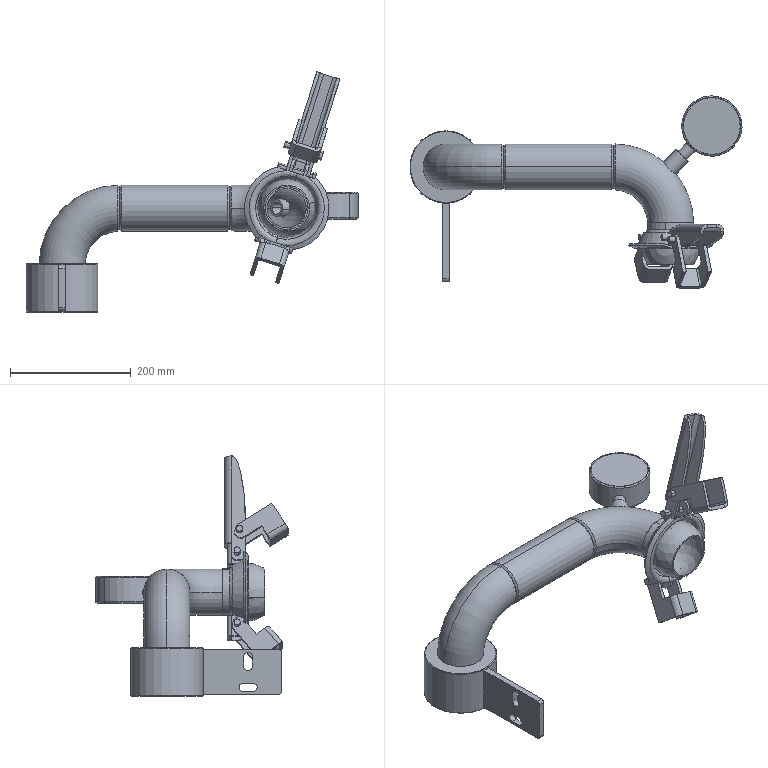Part | SolidWorks | features CompositeCurve 37 | 20 solids | 693 faces | box 550.016 x 318.498 x 397.435 mm | volume 1409303 mm3 | plane 405 | cylinder 139 | spline 85 | cone 34 | torus 26 | sphere 4 | commonest cylinder face diameters 10 x24 20 x12 14 x11 85 x10 6 x9 11 x8